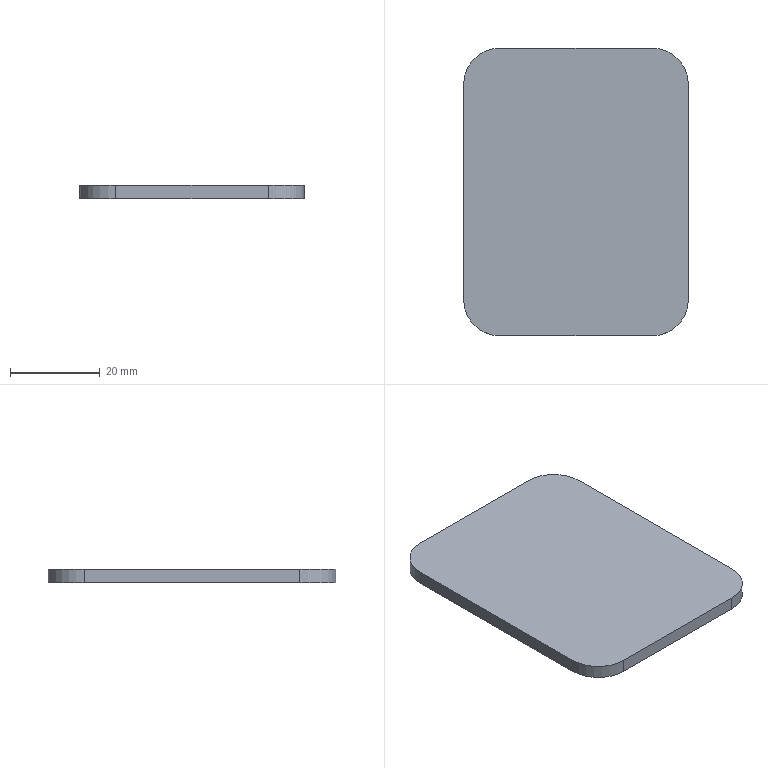Part | STEP file | Microwave Drying Flat Conveyor-CN2500x400-105-104 | 1 solid | 10 faces | box 50 x 64 x 3 mm | volume 9435 mm3 | plane 6 | cylinder 4 | commonest cylinder face diameters 16 x4
STEP:
#1=CARTESIAN_POINT('',(-25.,-24.,0.));
#2=VERTEX_POINT('',#1);
#3=CARTESIAN_POINT('',(-17.,-32.,0.));
#4=VERTEX_POINT('',#3);
#5=CARTESIAN_POINT('',(-17.,-24.,0.));
#6=DIRECTION('',(0.,0.,1.));
#7=DIRECTION('',(1.,0.,0.));
#8=AXIS2_PLACEMENT_3D('',#5,#6,#7);
#9=CIRCLE('',#8,8.);
#10=EDGE_CURVE('',#2,#4,#9,.T.);
#11=ORIENTED_EDGE('',*,*,#10,.T.);
#12=CARTESIAN_POINT('',(-17.,-32.,3.));
#13=VERTEX_POINT('',#12);
#14=CARTESIAN_POINT('',(-17.,-32.,3.));
#15=DIRECTION('',(0.,0.,-1.));
#16=VECTOR('',#15,1000.);
#17=LINE('',#14,#16);
#18=EDGE_CURVE('',#13,#4,#17,.T.);
#19=ORIENTED_EDGE('',*,*,#18,.F.);
#20=CARTESIAN_POINT('',(-25.,-24.,3.));
#21=VERTEX_POINT('',#20);
#22=CARTESIAN_POINT('',(-17.,-24.,3.));
#23=DIRECTION('',(0.,0.,1.));
#24=DIRECTION('',(1.,0.,0.));
#25=AXIS2_PLACEMENT_3D('',#22,#23,#24);
#26=CIRCLE('',#25,8.);
#27=EDGE_CURVE('',#21,#13,#26,.T.);
#28=ORIENTED_EDGE('',*,*,#27,.F.);
#29=CARTESIAN_POINT('',(-25.,-24.,3.));
#30=DIRECTION('',(0.,0.,-1.));
#31=VECTOR('',#30,1000.);
#32=LINE('',#29,#31);
#33=EDGE_CURVE('',#21,#2,#32,.T.);
#34=ORIENTED_EDGE('',*,*,#33,.T.);
#35=EDGE_LOOP('',(#11,#19,#28,#34));
#36=FACE_OUTER_BOUND('',#35,.T.);
#37=CARTESIAN_POINT('',(-17.,-24.,3.));
#38=DIRECTION('',(0.,0.,-1.));
#39=DIRECTION('',(-1.,0.,0.));
#40=AXIS2_PLACEMENT_3D('',#37,#38,#39);
#41=CYLINDRICAL_SURFACE('',#40,8.);
#42=ADVANCED_FACE('',(#36),#41,.T.);
#43=CARTESIAN_POINT('',(17.,-32.,0.));
#44=VERTEX_POINT('',#43);
#45=CARTESIAN_POINT('',(-17.,-32.,0.));
#46=DIRECTION('',(1.,0.,0.));
#47=VECTOR('',#46,1000.);
#48=LINE('',#45,#47);
#49=EDGE_CURVE('',#4,#44,#48,.T.);
#50=ORIENTED_EDGE('',*,*,#49,.T.);
#51=CARTESIAN_POINT('',(17.,-32.,3.));
#52=VERTEX_POINT('',#51);
#53=CARTESIAN_POINT('',(17.,-32.,3.));
#54=DIRECTION('',(0.,0.,-1.));
#55=VECTOR('',#54,1000.);
#56=LINE('',#53,#55);
#57=EDGE_CURVE('',#52,#44,#56,.T.);
#58=ORIENTED_EDGE('',*,*,#57,.F.);
#59=CARTESIAN_POINT('',(-17.,-32.,3.));
#60=DIRECTION('',(1.,0.,0.));
#61=VECTOR('',#60,1000.);
#62=LINE('',#59,#61);
#63=EDGE_CURVE('',#13,#52,#62,.T.);
#64=ORIENTED_EDGE('',*,*,#63,.F.);
#65=ORIENTED_EDGE('',*,*,#18,.T.);
#66=EDGE_LOOP('',(#50,#58,#64,#65));
#67=FACE_OUTER_BOUND('',#66,.T.);
#68=CARTESIAN_POINT('',(-17.,-32.,3.));
#69=DIRECTION('',(0.,1.,0.));
#70=DIRECTION('',(0.,0.,1.));
#71=AXIS2_PLACEMENT_3D('',#68,#69,#70);
#72=PLANE('',#71);
#73=ADVANCED_FACE('',(#67),#72,.F.);
#74=CARTESIAN_POINT('',(25.,-24.,0.));
#75=VERTEX_POINT('',#74);
#76=CARTESIAN_POINT('',(17.,-24.,0.));
#77=DIRECTION('',(0.,0.,1.));
#78=DIRECTION('',(1.,0.,0.));
#79=AXIS2_PLACEMENT_3D('',#76,#77,#78);
#80=CIRCLE('',#79,8.);
#81=EDGE_CURVE('',#44,#75,#80,.T.);
#82=ORIENTED_EDGE('',*,*,#81,.T.);
#83=CARTESIAN_POINT('',(25.,-24.,3.));
#84=VERTEX_POINT('',#83);
#85=CARTESIAN_POINT('',(25.,-24.,3.));
#86=DIRECTION('',(0.,0.,-1.));
#87=VECTOR('',#86,1000.);
#88=LINE('',#85,#87);
#89=EDGE_CURVE('',#84,#75,#88,.T.);
#90=ORIENTED_EDGE('',*,*,#89,.F.);
#91=CARTESIAN_POINT('',(17.,-24.,3.));
#92=DIRECTION('',(0.,0.,1.));
#93=DIRECTION('',(1.,0.,0.));
#94=AXIS2_PLACEMENT_3D('',#91,#92,#93);
#95=CIRCLE('',#94,8.);
#96=EDGE_CURVE('',#52,#84,#95,.T.);
#97=ORIENTED_EDGE('',*,*,#96,.F.);
#98=ORIENTED_EDGE('',*,*,#57,.T.);
#99=EDGE_LOOP('',(#82,#90,#97,#98));
#100=FACE_OUTER_BOUND('',#99,.T.);
#101=CARTESIAN_POINT('',(17.,-24.,3.));
#102=DIRECTION('',(0.,0.,-1.));
#103=DIRECTION('',(-1.,0.,0.));
#104=AXIS2_PLACEMENT_3D('',#101,#102,#103);
#105=CYLINDRICAL_SURFACE('',#104,8.);
#106=ADVANCED_FACE('',(#100),#105,.T.);
#107=CARTESIAN_POINT('',(25.,24.,0.));
#108=VERTEX_POINT('',#107);
#109=CARTESIAN_POINT('',(25.,24.,0.));
#110=DIRECTION('',(0.,1.,0.));
#111=VECTOR('',#110,1000.);
#112=LINE('',#109,#111);
#113=EDGE_CURVE('',#75,#108,#112,.T.);
#114=ORIENTED_EDGE('',*,*,#113,.T.);
#115=CARTESIAN_POINT('',(25.,24.,3.));
#116=VERTEX_POINT('',#115);
#117=CARTESIAN_POINT('',(25.,24.,3.));
#118=DIRECTION('',(0.,0.,-1.));
#119=VECTOR('',#118,1000.);
#120=LINE('',#117,#119);
#121=EDGE_CURVE('',#116,#108,#120,.T.);
#122=ORIENTED_EDGE('',*,*,#121,.F.);
#123=CARTESIAN_POINT('',(25.,24.,3.));
#124=DIRECTION('',(0.,1.,0.));
#125=VECTOR('',#124,1000.);
#126=LINE('',#123,#125);
#127=EDGE_CURVE('',#84,#116,#126,.T.);
#128=ORIENTED_EDGE('',*,*,#127,.F.);
#129=ORIENTED_EDGE('',*,*,#89,.T.);
#130=EDGE_LOOP('',(#114,#122,#128,#129));
#131=FACE_OUTER_BOUND('',#130,.T.);
#132=CARTESIAN_POINT('',(25.,24.,3.));
#133=DIRECTION('',(-1.,0.,0.));
#134=DIRECTION('',(0.,-1.,0.));
#135=AXIS2_PLACEMENT_3D('',#132,#133,#134);
#136=PLANE('',#135);
#137=ADVANCED_FACE('',(#131),#136,.F.);
#138=CARTESIAN_POINT('',(17.,32.,0.));
#139=VERTEX_POINT('',#138);
#140=CARTESIAN_POINT('',(17.,24.,0.));
#141=DIRECTION('',(0.,0.,1.));
#142=DIRECTION('',(-1.,0.,0.));
#143=AXIS2_PLACEMENT_3D('',#140,#141,#142);
#144=CIRCLE('',#143,8.);
#145=EDGE_CURVE('',#108,#139,#144,.T.);
#146=ORIENTED_EDGE('',*,*,#145,.T.);
#147=CARTESIAN_POINT('',(17.,32.,3.));
#148=VERTEX_POINT('',#147);
#149=CARTESIAN_POINT('',(17.,32.,3.));
#150=DIRECTION('',(0.,0.,-1.));
#151=VECTOR('',#150,1000.);
#152=LINE('',#149,#151);
#153=EDGE_CURVE('',#148,#139,#152,.T.);
#154=ORIENTED_EDGE('',*,*,#153,.F.);
#155=CARTESIAN_POINT('',(17.,24.,3.));
#156=DIRECTION('',(0.,0.,1.));
#157=DIRECTION('',(-1.,0.,0.));
#158=AXIS2_PLACEMENT_3D('',#155,#156,#157);
#159=CIRCLE('',#158,8.);
#160=EDGE_CURVE('',#116,#148,#159,.T.);
#161=ORIENTED_EDGE('',*,*,#160,.F.);
#162=ORIENTED_EDGE('',*,*,#121,.T.);
#163=EDGE_LOOP('',(#146,#154,#161,#162));
#164=FACE_OUTER_BOUND('',#163,.T.);
#165=CARTESIAN_POINT('',(17.,24.,3.));
#166=DIRECTION('',(0.,0.,-1.));
#167=DIRECTION('',(-1.,0.,0.));
#168=AXIS2_PLACEMENT_3D('',#165,#166,#167);
#169=CYLINDRICAL_SURFACE('',#168,8.);
#170=ADVANCED_FACE('',(#164),#169,.T.);
#171=CARTESIAN_POINT('',(-17.,32.,0.));
#172=VERTEX_POINT('',#171);
#173=CARTESIAN_POINT('',(-17.,32.,0.));
#174=DIRECTION('',(-1.,0.,0.));
#175=VECTOR('',#174,1000.);
#176=LINE('',#173,#175);
#177=EDGE_CURVE('',#139,#172,#176,.T.);
#178=ORIENTED_EDGE('',*,*,#177,.T.);
#179=CARTESIAN_POINT('',(-17.,32.,3.));
#180=VERTEX_POINT('',#179);
#181=CARTESIAN_POINT('',(-17.,32.,3.));
#182=DIRECTION('',(0.,0.,-1.));
#183=VECTOR('',#182,1000.);
#184=LINE('',#181,#183);
#185=EDGE_CURVE('',#180,#172,#184,.T.);
#186=ORIENTED_EDGE('',*,*,#185,.F.);
#187=CARTESIAN_POINT('',(-17.,32.,3.));
#188=DIRECTION('',(-1.,0.,0.));
#189=VECTOR('',#188,1000.);
#190=LINE('',#187,#189);
#191=EDGE_CURVE('',#148,#180,#190,.T.);
#192=ORIENTED_EDGE('',*,*,#191,.F.);
#193=ORIENTED_EDGE('',*,*,#153,.T.);
#194=EDGE_LOOP('',(#178,#186,#192,#193));
#195=FACE_OUTER_BOUND('',#194,.T.);
#196=CARTESIAN_POINT('',(-17.,32.,3.));
#197=DIRECTION('',(0.,-1.,0.));
#198=DIRECTION('',(0.,0.,-1.));
#199=AXIS2_PLACEMENT_3D('',#196,#197,#198);
#200=PLANE('',#199);
#201=ADVANCED_FACE('',(#195),#200,.F.);
#202=CARTESIAN_POINT('',(-25.,24.,0.));
#203=VERTEX_POINT('',#202);
#204=CARTESIAN_POINT('',(-17.,24.,0.));
#205=DIRECTION('',(0.,0.,1.));
#206=DIRECTION('',(1.,0.,0.));
#207=AXIS2_PLACEMENT_3D('',#204,#205,#206);
#208=CIRCLE('',#207,8.);
#209=EDGE_CURVE('',#172,#203,#208,.T.);
#210=ORIENTED_EDGE('',*,*,#209,.T.);
#211=CARTESIAN_POINT('',(-25.,24.,3.));
#212=VERTEX_POINT('',#211);
#213=CARTESIAN_POINT('',(-25.,24.,3.));
#214=DIRECTION('',(0.,0.,-1.));
#215=VECTOR('',#214,1000.);
#216=LINE('',#213,#215);
#217=EDGE_CURVE('',#212,#203,#216,.T.);
#218=ORIENTED_EDGE('',*,*,#217,.F.);
#219=CARTESIAN_POINT('',(-17.,24.,3.));
#220=DIRECTION('',(0.,0.,1.));
#221=DIRECTION('',(1.,0.,0.));
#222=AXIS2_PLACEMENT_3D('',#219,#220,#221);
#223=CIRCLE('',#222,8.);
#224=EDGE_CURVE('',#180,#212,#223,.T.);
#225=ORIENTED_EDGE('',*,*,#224,.F.);
#226=ORIENTED_EDGE('',*,*,#185,.T.);
#227=EDGE_LOOP('',(#210,#218,#225,#226));
#228=FACE_OUTER_BOUND('',#227,.T.);
#229=CARTESIAN_POINT('',(-17.,24.,3.));
#230=DIRECTION('',(0.,0.,-1.));
#231=DIRECTION('',(-1.,0.,0.));
#232=AXIS2_PLACEMENT_3D('',#229,#230,#231);
#233=CYLINDRICAL_SURFACE('',#232,8.);
#234=ADVANCED_FACE('',(#228),#233,.T.);
#235=CARTESIAN_POINT('',(-25.,24.,0.));
#236=DIRECTION('',(0.,-1.,0.));
#237=VECTOR('',#236,1000.);
#238=LINE('',#235,#237);
#239=EDGE_CURVE('',#203,#2,#238,.T.);
#240=ORIENTED_EDGE('',*,*,#239,.T.);
#241=ORIENTED_EDGE('',*,*,#33,.F.);
#242=CARTESIAN_POINT('',(-25.,24.,3.));
#243=DIRECTION('',(0.,-1.,0.));
#244=VECTOR('',#243,1000.);
#245=LINE('',#242,#244);
#246=EDGE_CURVE('',#212,#21,#245,.T.);
#247=ORIENTED_EDGE('',*,*,#246,.F.);
#248=ORIENTED_EDGE('',*,*,#217,.T.);
#249=EDGE_LOOP('',(#240,#241,#247,#248));
#250=FACE_OUTER_BOUND('',#249,.T.);
#251=CARTESIAN_POINT('',(-25.,24.,3.));
#252=DIRECTION('',(1.,0.,0.));
#253=DIRECTION('',(0.,1.,0.));
#254=AXIS2_PLACEMENT_3D('',#251,#252,#253);
#255=PLANE('',#254);
#256=ADVANCED_FACE('',(#250),#255,.F.);
#257=ORIENTED_EDGE('',*,*,#27,.T.);
#258=ORIENTED_EDGE('',*,*,#63,.T.);
#259=ORIENTED_EDGE('',*,*,#96,.T.);
#260=ORIENTED_EDGE('',*,*,#127,.T.);
#261=ORIENTED_EDGE('',*,*,#160,.T.);
#262=ORIENTED_EDGE('',*,*,#191,.T.);
#263=ORIENTED_EDGE('',*,*,#224,.T.);
#264=ORIENTED_EDGE('',*,*,#246,.T.);
#265=EDGE_LOOP('',(#257,#258,#259,#260,#261,#262,#263,#264));
#266=FACE_OUTER_BOUND('',#265,.T.);
#267=CARTESIAN_POINT('',(-17.,-24.,3.));
#268=DIRECTION('',(0.,0.,1.));
#269=DIRECTION('',(1.,0.,0.));
#270=AXIS2_PLACEMENT_3D('',#267,#268,#269);
#271=PLANE('',#270);
#272=ADVANCED_FACE('',(#266),#271,.T.);
#273=ORIENTED_EDGE('',*,*,#10,.F.);
#274=ORIENTED_EDGE('',*,*,#239,.F.);
#275=ORIENTED_EDGE('',*,*,#209,.F.);
#276=ORIENTED_EDGE('',*,*,#177,.F.);
#277=ORIENTED_EDGE('',*,*,#145,.F.);
#278=ORIENTED_EDGE('',*,*,#113,.F.);
#279=ORIENTED_EDGE('',*,*,#81,.F.);
#280=ORIENTED_EDGE('',*,*,#49,.F.);
#281=EDGE_LOOP('',(#273,#274,#275,#276,#277,#278,#279,#280));
#282=FACE_OUTER_BOUND('',#281,.T.);
#283=CARTESIAN_POINT('',(-17.,-24.,0.));
#284=DIRECTION('',(0.,0.,1.));
#285=DIRECTION('',(1.,0.,0.));
#286=AXIS2_PLACEMENT_3D('',#283,#284,#285);
#287=PLANE('',#286);
#288=ADVANCED_FACE('',(#282),#287,.F.);
#289=CLOSED_SHELL('',(#42,#73,#106,#137,#170,#201,#234,#256,#272,#288));
#290=MANIFOLD_SOLID_BREP('',#289);
#291=CARTESIAN_POINT('',(0.,0.,0.));
#292=DIRECTION('',(0.,0.,1.));
#293=DIRECTION('',(1.,0.,0.));
#294=AXIS2_PLACEMENT_3D('',#291,#292,#293);
#295=(LENGTH_UNIT()NAMED_UNIT(*)SI_UNIT(.MILLI.,.METRE.));
#296=UNCERTAINTY_MEASURE_WITH_UNIT(LENGTH_MEASURE(0.00001),#295,'','');
#297=(NAMED_UNIT(*)PLANE_ANGLE_UNIT()SI_UNIT($,.RADIAN.));
#298=(NAMED_UNIT(*)SI_UNIT($,.STERADIAN.)SOLID_ANGLE_UNIT());
#299=(GEOMETRIC_REPRESENTATION_CONTEXT(3)GLOBAL_UNCERTAINTY_ASSIGNED_CONTEXT((#296))GLOBAL_UNIT_ASSIGNED_CONTEXT((#295,#297,#298))REPRESENTATION_CONTEXT('',''));
#300=ADVANCED_BREP_SHAPE_REPRESENTATION('',(#290,#294),#299);